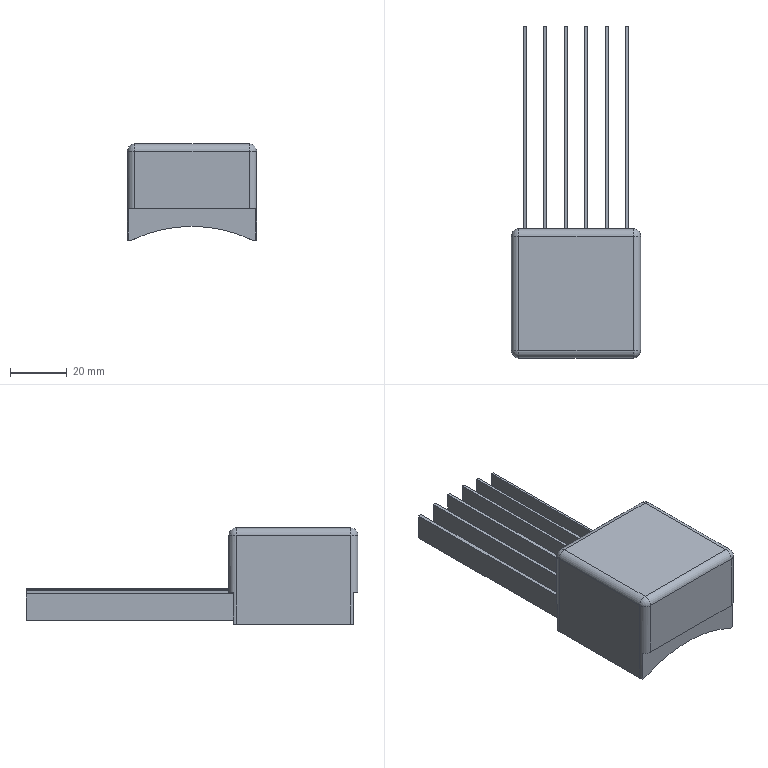Part | SolidWorks | features BaseBody 1 | 1 solid | 57 faces | box 45.408 x 116.688 x 33.872 mm | volume 65935 mm3 | plane 37 | cylinder 16 | sphere 4 | commonest cylinder face diameters 5.28 x8 165.792 x6 97.2 x2